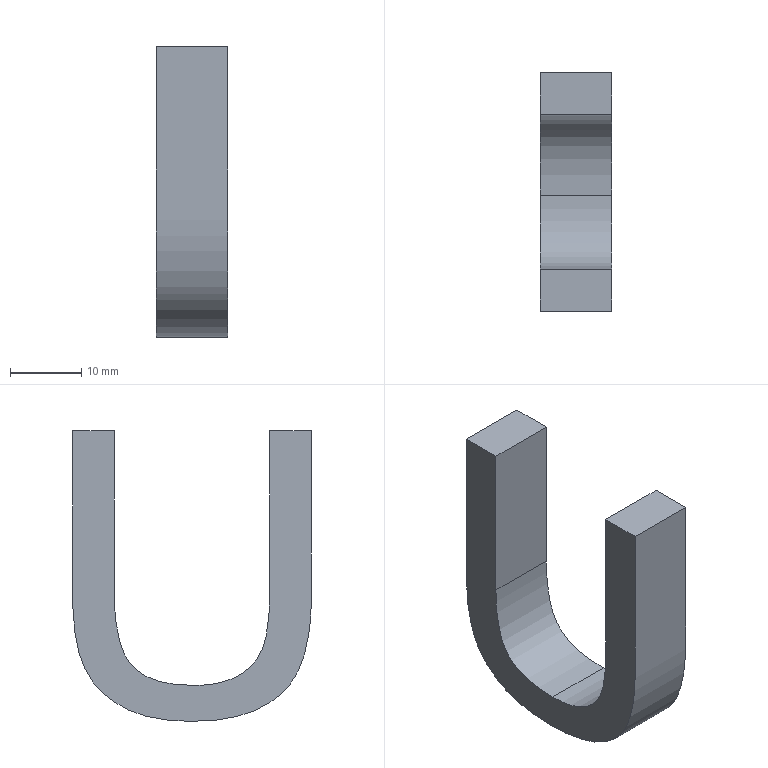Part | NX | features solid 2 | 1 solid | 8 faces | box 10 x 33.468 x 40.78 mm | volume 5118 mm3 | plane 5 | spline 3
STEP:
#1=CARTESIAN_POINT('',(2250.,262.21,377.01));
#2=VERTEX_POINT('',#1);
#3=CARTESIAN_POINT('',(2250.,262.21,400.));
#4=VERTEX_POINT('',#3);
#5=CARTESIAN_POINT('',(2250.,262.21,377.01));
#6=CARTESIAN_POINT('',(2250.,262.21,384.673));
#7=CARTESIAN_POINT('',(2250.,262.21,392.337));
#8=CARTESIAN_POINT('',(2250.,262.21,400.));
#9=B_SPLINE_CURVE_WITH_KNOTS('',3,(#5,#6,#7,#8),.UNSPECIFIED.,.F.,.F.,(4,4),(0.,0.1078),.PIECEWISE_BEZIER_KNOTS.);
#10=EDGE_CURVE('',#2,#4,#9,.T.);
#11=ORIENTED_EDGE('',*,*,#10,.F.);
#12=CARTESIAN_POINT('',(2260.,262.21,377.01));
#13=VERTEX_POINT('',#12);
#14=CARTESIAN_POINT('',(2260.,262.21,377.01));
#15=DIRECTION('',(-1.,0.,0.));
#16=VECTOR('',#15,1000.);
#17=LINE('',#14,#16);
#18=EDGE_CURVE('',#13,#2,#17,.T.);
#19=ORIENTED_EDGE('',*,*,#18,.F.);
#20=CARTESIAN_POINT('',(2260.,262.21,400.));
#21=VERTEX_POINT('',#20);
#22=CARTESIAN_POINT('',(2260.,262.21,377.01));
#23=CARTESIAN_POINT('',(2260.,262.21,384.673));
#24=CARTESIAN_POINT('',(2260.,262.21,392.337));
#25=CARTESIAN_POINT('',(2260.,262.21,400.));
#26=B_SPLINE_CURVE_WITH_KNOTS('',3,(#22,#23,#24,#25),.UNSPECIFIED.,.F.,.F.,(4,4),(0.,0.1078),.PIECEWISE_BEZIER_KNOTS.);
#27=EDGE_CURVE('',#13,#21,#26,.T.);
#28=ORIENTED_EDGE('',*,*,#27,.T.);
#29=CARTESIAN_POINT('',(2260.,262.21,400.));
#30=DIRECTION('',(-1.,0.,0.));
#31=VECTOR('',#30,1000.);
#32=LINE('',#29,#31);
#33=EDGE_CURVE('',#21,#4,#32,.T.);
#34=ORIENTED_EDGE('',*,*,#33,.T.);
#35=EDGE_LOOP('',(#11,#19,#28,#34));
#36=FACE_BOUND('',#35,.T.);
#37=CARTESIAN_POINT('',(2260.,262.21,377.01));
#38=DIRECTION('',(0.,-1.,0.));
#39=DIRECTION('',(0.,0.,-1.));
#40=AXIS2_PLACEMENT_3D('',#37,#38,#39);
#41=PLANE('',#40);
#42=ADVANCED_FACE('',(#36),#41,.T.);
#43=CARTESIAN_POINT('',(2250.,268.068,400.));
#44=VERTEX_POINT('',#43);
#45=CARTESIAN_POINT('',(2250.,262.21,400.));
#46=CARTESIAN_POINT('',(2250.,264.163,400.));
#47=CARTESIAN_POINT('',(2250.,266.116,400.));
#48=CARTESIAN_POINT('',(2250.,268.068,400.));
#49=B_SPLINE_CURVE_WITH_KNOTS('',3,(#45,#46,#47,#48),.UNSPECIFIED.,.F.,.F.,(4,4),(0.1078,0.1353),.PIECEWISE_BEZIER_KNOTS.);
#50=EDGE_CURVE('',#4,#44,#49,.T.);
#51=ORIENTED_EDGE('',*,*,#50,.F.);
#52=ORIENTED_EDGE('',*,*,#33,.F.);
#53=CARTESIAN_POINT('',(2260.,268.068,400.));
#54=VERTEX_POINT('',#53);
#55=CARTESIAN_POINT('',(2260.,262.21,400.));
#56=CARTESIAN_POINT('',(2260.,264.163,400.));
#57=CARTESIAN_POINT('',(2260.,266.116,400.));
#58=CARTESIAN_POINT('',(2260.,268.068,400.));
#59=B_SPLINE_CURVE_WITH_KNOTS('',3,(#55,#56,#57,#58),.UNSPECIFIED.,.F.,.F.,(4,4),(0.1078,0.1353),.PIECEWISE_BEZIER_KNOTS.);
#60=EDGE_CURVE('',#21,#54,#59,.T.);
#61=ORIENTED_EDGE('',*,*,#60,.T.);
#62=CARTESIAN_POINT('',(2260.,268.068,400.));
#63=DIRECTION('',(-1.,0.,0.));
#64=VECTOR('',#63,1000.);
#65=LINE('',#62,#64);
#66=EDGE_CURVE('',#54,#44,#65,.T.);
#67=ORIENTED_EDGE('',*,*,#66,.T.);
#68=EDGE_LOOP('',(#51,#52,#61,#67));
#69=FACE_BOUND('',#68,.T.);
#70=CARTESIAN_POINT('',(2260.,262.21,400.));
#71=DIRECTION('',(0.,0.,1.));
#72=DIRECTION('',(1.,0.,0.));
#73=AXIS2_PLACEMENT_3D('',#70,#71,#72);
#74=PLANE('',#73);
#75=ADVANCED_FACE('',(#69),#74,.T.);
#76=CARTESIAN_POINT('',(2250.,234.6,400.));
#77=VERTEX_POINT('',#76);
#78=CARTESIAN_POINT('',(2250.,268.068,400.));
#79=CARTESIAN_POINT('',(2250.,268.068,392.27));
#80=CARTESIAN_POINT('',(2250.,268.068,384.54));
#81=CARTESIAN_POINT('',(2250.,268.068,372.757));
#82=CARTESIAN_POINT('',(2250.,267.594,369.56));
#83=CARTESIAN_POINT('',(2250.,265.654,364.817));
#84=CARTESIAN_POINT('',(2250.,263.908,362.876));
#85=CARTESIAN_POINT('',(2250.,261.379,361.404));
#86=CARTESIAN_POINT('',(2250.,258.86,359.939));
#87=CARTESIAN_POINT('',(2250.,255.541,359.22));
#88=CARTESIAN_POINT('',(2250.,247.464,359.22));
#89=CARTESIAN_POINT('',(2250.,244.191,359.847));
#90=CARTESIAN_POINT('',(2250.,239.131,362.423));
#91=CARTESIAN_POINT('',(2250.,237.323,364.283));
#92=CARTESIAN_POINT('',(2250.,235.142,369.189));
#93=CARTESIAN_POINT('',(2250.,234.6,372.543));
#94=CARTESIAN_POINT('',(2250.,234.6,384.54));
#95=CARTESIAN_POINT('',(2250.,234.6,392.27));
#96=CARTESIAN_POINT('',(2250.,234.6,400.));
#97=B_SPLINE_CURVE_WITH_KNOTS('',3,(#78,#79,#80,#81,#82,#83,#84,#85,#86,#87,#88,#89,#90,#91,#92,#93,#94,#95,#96),.UNSPECIFIED.,.F.,.F.,(4,2,2,3,2,2,2,2,4),(0.1353,0.244,0.3011,0.3589,0.4118,0.4631,0.5147,0.5652,0.6568),.UNSPECIFIED.);
#98=EDGE_CURVE('',#44,#77,#97,.T.);
#99=ORIENTED_EDGE('',*,*,#98,.F.);
#100=ORIENTED_EDGE('',*,*,#66,.F.);
#101=CARTESIAN_POINT('',(2260.,234.6,400.));
#102=VERTEX_POINT('',#101);
#103=CARTESIAN_POINT('',(2260.,268.068,400.));
#104=CARTESIAN_POINT('',(2260.,268.068,392.27));
#105=CARTESIAN_POINT('',(2260.,268.068,384.54));
#106=CARTESIAN_POINT('',(2260.,268.068,372.757));
#107=CARTESIAN_POINT('',(2260.,267.594,369.56));
#108=CARTESIAN_POINT('',(2260.,265.654,364.817));
#109=CARTESIAN_POINT('',(2260.,263.908,362.876));
#110=CARTESIAN_POINT('',(2260.,261.379,361.404));
#111=CARTESIAN_POINT('',(2260.,258.86,359.939));
#112=CARTESIAN_POINT('',(2260.,255.541,359.22));
#113=CARTESIAN_POINT('',(2260.,247.464,359.22));
#114=CARTESIAN_POINT('',(2260.,244.191,359.847));
#115=CARTESIAN_POINT('',(2260.,239.131,362.423));
#116=CARTESIAN_POINT('',(2260.,237.323,364.283));
#117=CARTESIAN_POINT('',(2260.,235.142,369.189));
#118=CARTESIAN_POINT('',(2260.,234.6,372.543));
#119=CARTESIAN_POINT('',(2260.,234.6,384.54));
#120=CARTESIAN_POINT('',(2260.,234.6,392.27));
#121=CARTESIAN_POINT('',(2260.,234.6,400.));
#122=B_SPLINE_CURVE_WITH_KNOTS('',3,(#103,#104,#105,#106,#107,#108,#109,#110,#111,#112,#113,#114,#115,#116,#117,#118,#119,#120,#121),.UNSPECIFIED.,.F.,.F.,(4,2,2,3,2,2,2,2,4),(0.1353,0.244,0.3011,0.3589,0.4118,0.4631,0.5147,0.5652,0.6568),.UNSPECIFIED.);
#123=EDGE_CURVE('',#54,#102,#122,.T.);
#124=ORIENTED_EDGE('',*,*,#123,.T.);
#125=CARTESIAN_POINT('',(2260.,234.6,400.));
#126=DIRECTION('',(-1.,0.,0.));
#127=VECTOR('',#126,1000.);
#128=LINE('',#125,#127);
#129=EDGE_CURVE('',#102,#77,#128,.T.);
#130=ORIENTED_EDGE('',*,*,#129,.T.);
#131=EDGE_LOOP('',(#99,#100,#124,#130));
#132=FACE_BOUND('',#131,.T.);
#133=CARTESIAN_POINT('',(2260.,268.068,400.));
#134=CARTESIAN_POINT('',(2250.,268.068,400.));
#135=CARTESIAN_POINT('',(2260.,268.068,397.683));
#136=CARTESIAN_POINT('',(2250.,268.068,397.683));
#137=CARTESIAN_POINT('',(2260.,268.067,393.052));
#138=CARTESIAN_POINT('',(2250.,268.067,393.052));
#139=CARTESIAN_POINT('',(2260.,268.073,386.091));
#140=CARTESIAN_POINT('',(2250.,268.073,386.091));
#141=CARTESIAN_POINT('',(2260.,268.054,380.332));
#142=CARTESIAN_POINT('',(2250.,268.054,380.332));
#143=CARTESIAN_POINT('',(2260.,268.093,375.632));
#144=CARTESIAN_POINT('',(2250.,268.093,375.632));
#145=CARTESIAN_POINT('',(2260.,267.838,371.45));
#146=CARTESIAN_POINT('',(2250.,267.838,371.45));
#147=CARTESIAN_POINT('',(2260.,267.121,368.135));
#148=CARTESIAN_POINT('',(2250.,267.121,368.135));
#149=CARTESIAN_POINT('',(2260.,265.887,365.578));
#150=CARTESIAN_POINT('',(2250.,265.887,365.578));
#151=CARTESIAN_POINT('',(2260.,264.566,363.831));
#152=CARTESIAN_POINT('',(2250.,264.566,363.831));
#153=CARTESIAN_POINT('',(2260.,262.884,362.329));
#154=CARTESIAN_POINT('',(2250.,262.884,362.329));
#155=CARTESIAN_POINT('',(2260.,260.817,360.993));
#156=CARTESIAN_POINT('',(2250.,260.817,360.993));
#157=CARTESIAN_POINT('',(2260.,258.084,359.941));
#158=CARTESIAN_POINT('',(2250.,258.084,359.941));
#159=CARTESIAN_POINT('',(2260.,254.99,359.343));
#160=CARTESIAN_POINT('',(2250.,254.99,359.343));
#161=CARTESIAN_POINT('',(2260.,251.302,359.155));
#162=CARTESIAN_POINT('',(2250.,251.302,359.155));
#163=CARTESIAN_POINT('',(2260.,246.456,359.428));
#164=CARTESIAN_POINT('',(2250.,246.456,359.428));
#165=CARTESIAN_POINT('',(2260.,241.665,360.738));
#166=CARTESIAN_POINT('',(2250.,241.665,360.738));
#167=CARTESIAN_POINT('',(2260.,237.61,363.842));
#168=CARTESIAN_POINT('',(2250.,237.61,363.842));
#169=CARTESIAN_POINT('',(2260.,235.713,367.487));
#170=CARTESIAN_POINT('',(2250.,235.713,367.487));
#171=CARTESIAN_POINT('',(2260.,234.866,371.555));
#172=CARTESIAN_POINT('',(2250.,234.866,371.555));
#173=CARTESIAN_POINT('',(2260.,234.568,375.18));
#174=CARTESIAN_POINT('',(2250.,234.568,375.18));
#175=CARTESIAN_POINT('',(2260.,234.608,379.375));
#176=CARTESIAN_POINT('',(2250.,234.608,379.375));
#177=CARTESIAN_POINT('',(2260.,234.595,384.857));
#178=CARTESIAN_POINT('',(2250.,234.595,384.857));
#179=CARTESIAN_POINT('',(2260.,234.602,391.747));
#180=CARTESIAN_POINT('',(2250.,234.602,391.747));
#181=CARTESIAN_POINT('',(2260.,234.6,397.248));
#182=CARTESIAN_POINT('',(2250.,234.6,397.248));
#183=CARTESIAN_POINT('',(2260.,234.6,400.));
#184=CARTESIAN_POINT('',(2250.,234.6,400.));
#185=B_SPLINE_SURFACE_WITH_KNOTS('',3,1,((#133,#134),(#135,#136),(#137,#138),(#139,#140),(#141,#142),(#143,#144),(#145,#146),(#147,#148),(#149,#150),(#151,#152),(#153,#154),(#155,#156),(#157,#158),(#159,#160),(#161,#162),(#163,#164),(#165,#166),(#167,#168),(#169,#170),(#171,#172),(#173,#174),(#175,#176),(#177,#178),(#179,#180),(#181,#182),(#183,#184)),.SURF_OF_LINEAR_EXTRUSION.,.F.,.F.,.F.,(4,1,1,1,1,1,1,1,1,1,1,1,1,1,1,1,1,1,1,1,1,1,1,4),(2,2),(0.1353,0.1679,0.2005,0.2331,0.2494,0.2657,0.2983,0.3146,0.3309,0.3471,0.3634,0.3797,0.396,0.4123,0.4286,0.4612,0.4938,0.5264,0.5427,0.559,0.5753,0.5916,0.6242,0.6568),(0.,1.),.UNSPECIFIED.);
#186=ADVANCED_FACE('',(#132),#185,.T.);
#187=CARTESIAN_POINT('',(2250.,240.459,400.));
#188=VERTEX_POINT('',#187);
#189=CARTESIAN_POINT('',(2250.,234.6,400.));
#190=CARTESIAN_POINT('',(2250.,236.553,400.));
#191=CARTESIAN_POINT('',(2250.,238.506,400.));
#192=CARTESIAN_POINT('',(2250.,240.459,400.));
#193=B_SPLINE_CURVE_WITH_KNOTS('',3,(#189,#190,#191,#192),.UNSPECIFIED.,.F.,.F.,(4,4),(0.6568,0.686),.PIECEWISE_BEZIER_KNOTS.);
#194=EDGE_CURVE('',#77,#188,#193,.T.);
#195=ORIENTED_EDGE('',*,*,#194,.F.);
#196=ORIENTED_EDGE('',*,*,#129,.F.);
#197=CARTESIAN_POINT('',(2260.,240.459,400.));
#198=VERTEX_POINT('',#197);
#199=CARTESIAN_POINT('',(2260.,234.6,400.));
#200=CARTESIAN_POINT('',(2260.,236.553,400.));
#201=CARTESIAN_POINT('',(2260.,238.506,400.));
#202=CARTESIAN_POINT('',(2260.,240.459,400.));
#203=B_SPLINE_CURVE_WITH_KNOTS('',3,(#199,#200,#201,#202),.UNSPECIFIED.,.F.,.F.,(4,4),(0.6568,0.686),.PIECEWISE_BEZIER_KNOTS.);
#204=EDGE_CURVE('',#102,#198,#203,.T.);
#205=ORIENTED_EDGE('',*,*,#204,.T.);
#206=CARTESIAN_POINT('',(2260.,240.459,400.));
#207=DIRECTION('',(-1.,0.,0.));
#208=VECTOR('',#207,1000.);
#209=LINE('',#206,#208);
#210=EDGE_CURVE('',#198,#188,#209,.T.);
#211=ORIENTED_EDGE('',*,*,#210,.T.);
#212=EDGE_LOOP('',(#195,#196,#205,#211));
#213=FACE_BOUND('',#212,.T.);
#214=CARTESIAN_POINT('',(2260.,234.6,400.));
#215=DIRECTION('',(0.,0.,1.));
#216=DIRECTION('',(1.,0.,0.));
#217=AXIS2_PLACEMENT_3D('',#214,#215,#216);
#218=PLANE('',#217);
#219=ADVANCED_FACE('',(#213),#218,.T.);
#220=CARTESIAN_POINT('',(2250.,250.937,364.268));
#221=VERTEX_POINT('',#220);
#222=CARTESIAN_POINT('',(2250.,240.459,400.));
#223=CARTESIAN_POINT('',(2250.,240.459,392.337));
#224=CARTESIAN_POINT('',(2250.,240.459,384.673));
#225=CARTESIAN_POINT('',(2250.,240.459,373.537));
#226=CARTESIAN_POINT('',(2250.,240.795,370.983));
#227=CARTESIAN_POINT('',(2250.,241.471,369.356));
#228=CARTESIAN_POINT('',(2250.,242.156,367.709));
#229=CARTESIAN_POINT('',(2250.,243.304,366.455));
#230=CARTESIAN_POINT('',(2250.,246.583,364.692));
#231=CARTESIAN_POINT('',(2250.,248.581,364.237));
#232=CARTESIAN_POINT('',(2250.,250.937,364.268));
#233=B_SPLINE_CURVE_WITH_KNOTS('',3,(#222,#223,#224,#225,#226,#227,#228,#229,#230,#231,#232),.UNSPECIFIED.,.F.,.F.,(4,2,3,2,4),(0.686,0.8008,0.8528,0.8793,0.9064),.UNSPECIFIED.);
#234=EDGE_CURVE('',#188,#221,#233,.T.);
#235=ORIENTED_EDGE('',*,*,#234,.F.);
#236=ORIENTED_EDGE('',*,*,#210,.F.);
#237=CARTESIAN_POINT('',(2260.,250.937,364.268));
#238=VERTEX_POINT('',#237);
#239=CARTESIAN_POINT('',(2260.,240.459,400.));
#240=CARTESIAN_POINT('',(2260.,240.459,392.337));
#241=CARTESIAN_POINT('',(2260.,240.459,384.673));
#242=CARTESIAN_POINT('',(2260.,240.459,373.537));
#243=CARTESIAN_POINT('',(2260.,240.795,370.983));
#244=CARTESIAN_POINT('',(2260.,241.471,369.356));
#245=CARTESIAN_POINT('',(2260.,242.156,367.709));
#246=CARTESIAN_POINT('',(2260.,243.304,366.455));
#247=CARTESIAN_POINT('',(2260.,246.583,364.692));
#248=CARTESIAN_POINT('',(2260.,248.581,364.237));
#249=CARTESIAN_POINT('',(2260.,250.937,364.268));
#250=B_SPLINE_CURVE_WITH_KNOTS('',3,(#239,#240,#241,#242,#243,#244,#245,#246,#247,#248,#249),.UNSPECIFIED.,.F.,.F.,(4,2,3,2,4),(0.686,0.8008,0.8528,0.8793,0.9064),.UNSPECIFIED.);
#251=EDGE_CURVE('',#198,#238,#250,.T.);
#252=ORIENTED_EDGE('',*,*,#251,.T.);
#253=CARTESIAN_POINT('',(2260.,250.937,364.268));
#254=DIRECTION('',(-1.,0.,0.));
#255=VECTOR('',#254,1000.);
#256=LINE('',#253,#255);
#257=EDGE_CURVE('',#238,#221,#256,.T.);
#258=ORIENTED_EDGE('',*,*,#257,.T.);
#259=EDGE_LOOP('',(#235,#236,#252,#258));
#260=FACE_BOUND('',#259,.T.);
#261=CARTESIAN_POINT('',(2260.,240.459,400.));
#262=CARTESIAN_POINT('',(2250.,240.459,400.));
#263=CARTESIAN_POINT('',(2260.,240.459,398.161));
#264=CARTESIAN_POINT('',(2250.,240.459,398.161));
#265=CARTESIAN_POINT('',(2260.,240.459,394.484));
#266=CARTESIAN_POINT('',(2250.,240.459,394.484));
#267=CARTESIAN_POINT('',(2260.,240.458,388.967));
#268=CARTESIAN_POINT('',(2250.,240.458,388.967));
#269=CARTESIAN_POINT('',(2260.,240.459,383.453));
#270=CARTESIAN_POINT('',(2250.,240.459,383.453));
#271=CARTESIAN_POINT('',(2260.,240.456,378.849));
#272=CARTESIAN_POINT('',(2250.,240.456,378.849));
#273=CARTESIAN_POINT('',(2260.,240.462,375.187));
#274=CARTESIAN_POINT('',(2250.,240.462,375.187));
#275=CARTESIAN_POINT('',(2260.,240.604,373.276));
#276=CARTESIAN_POINT('',(2250.,240.604,373.276));
#277=CARTESIAN_POINT('',(2260.,240.785,371.929));
#278=CARTESIAN_POINT('',(2250.,240.785,371.929));
#279=CARTESIAN_POINT('',(2260.,240.956,371.019));
#280=CARTESIAN_POINT('',(2250.,240.956,371.019));
#281=CARTESIAN_POINT('',(2260.,241.13,370.338));
#282=CARTESIAN_POINT('',(2250.,241.13,370.338));
#283=CARTESIAN_POINT('',(2260.,241.283,369.85));
#284=CARTESIAN_POINT('',(2250.,241.283,369.85));
#285=CARTESIAN_POINT('',(2260.,241.395,369.545));
#286=CARTESIAN_POINT('',(2250.,241.395,369.545));
#287=CARTESIAN_POINT('',(2260.,241.467,369.361));
#288=CARTESIAN_POINT('',(2250.,241.467,369.361));
#289=CARTESIAN_POINT('',(2260.,241.679,368.88));
#290=CARTESIAN_POINT('',(2250.,241.679,368.88));
#291=CARTESIAN_POINT('',(2260.,242.034,368.217));
#292=CARTESIAN_POINT('',(2250.,242.034,368.217));
#293=CARTESIAN_POINT('',(2260.,242.946,366.927));
#294=CARTESIAN_POINT('',(2250.,242.946,366.927));
#295=CARTESIAN_POINT('',(2260.,244.726,365.527));
#296=CARTESIAN_POINT('',(2250.,244.726,365.527));
#297=CARTESIAN_POINT('',(2260.,247.533,364.47));
#298=CARTESIAN_POINT('',(2250.,247.533,364.47));
#299=CARTESIAN_POINT('',(2260.,249.738,364.252));
#300=CARTESIAN_POINT('',(2250.,249.738,364.252));
#301=CARTESIAN_POINT('',(2260.,250.937,364.268));
#302=CARTESIAN_POINT('',(2250.,250.937,364.268));
#303=B_SPLINE_SURFACE_WITH_KNOTS('',3,1,((#261,#262),(#263,#264),(#265,#266),(#267,#268),(#269,#270),(#271,#272),(#273,#274),(#275,#276),(#277,#278),(#279,#280),(#281,#282),(#283,#284),(#285,#286),(#287,#288),(#289,#290),(#291,#292),(#293,#294),(#295,#296),(#297,#298),(#299,#300),(#301,#302)),.SURF_OF_LINEAR_EXTRUSION.,.F.,.F.,.F.,(4,1,1,1,1,1,1,1,1,1,1,1,1,1,1,1,1,1,4),(2,2),(0.686,0.7136,0.7411,0.7687,0.7962,0.81,0.8237,0.8306,0.8375,0.8444,0.8478,0.8513,0.853,0.8547,0.8582,0.8651,0.8788,0.8926,0.9064),(0.,1.),.UNSPECIFIED.);
#304=ADVANCED_FACE('',(#260),#303,.T.);
#305=CARTESIAN_POINT('',(2250.,250.937,364.268));
#306=CARTESIAN_POINT('',(2250.,255.021,364.237));
#307=CARTESIAN_POINT('',(2250.,257.896,365.109));
#308=CARTESIAN_POINT('',(2250.,261.338,368.642));
#309=CARTESIAN_POINT('',(2250.,262.21,372.008));
#310=CARTESIAN_POINT('',(2250.,262.21,377.01));
#311=B_SPLINE_CURVE_WITH_KNOTS('',3,(#305,#306,#307,#308,#309,#310),.UNSPECIFIED.,.F.,.F.,(4,2,4),(0.9064,0.9534,1.),.UNSPECIFIED.);
#312=EDGE_CURVE('',#221,#2,#311,.T.);
#313=ORIENTED_EDGE('',*,*,#312,.F.);
#314=ORIENTED_EDGE('',*,*,#257,.F.);
#315=CARTESIAN_POINT('',(2260.,250.937,364.268));
#316=CARTESIAN_POINT('',(2260.,255.021,364.237));
#317=CARTESIAN_POINT('',(2260.,257.896,365.109));
#318=CARTESIAN_POINT('',(2260.,261.338,368.642));
#319=CARTESIAN_POINT('',(2260.,262.21,372.008));
#320=CARTESIAN_POINT('',(2260.,262.21,377.01));
#321=B_SPLINE_CURVE_WITH_KNOTS('',3,(#315,#316,#317,#318,#319,#320),.UNSPECIFIED.,.F.,.F.,(4,2,4),(0.9064,0.9534,1.),.UNSPECIFIED.);
#322=EDGE_CURVE('',#238,#13,#321,.T.);
#323=ORIENTED_EDGE('',*,*,#322,.T.);
#324=ORIENTED_EDGE('',*,*,#18,.T.);
#325=EDGE_LOOP('',(#313,#314,#323,#324));
#326=FACE_BOUND('',#325,.T.);
#327=CARTESIAN_POINT('',(2260.,250.937,364.268));
#328=CARTESIAN_POINT('',(2250.,250.937,364.268));
#329=CARTESIAN_POINT('',(2260.,252.97,364.252));
#330=CARTESIAN_POINT('',(2250.,252.97,364.252));
#331=CARTESIAN_POINT('',(2260.,255.569,364.562));
#332=CARTESIAN_POINT('',(2250.,255.569,364.562));
#333=CARTESIAN_POINT('',(2260.,258.164,365.659));
#334=CARTESIAN_POINT('',(2250.,258.164,365.659));
#335=CARTESIAN_POINT('',(2260.,259.665,366.783));
#336=CARTESIAN_POINT('',(2250.,259.665,366.783));
#337=CARTESIAN_POINT('',(2260.,260.79,368.371));
#338=CARTESIAN_POINT('',(2250.,260.79,368.371));
#339=CARTESIAN_POINT('',(2260.,261.882,371.353));
#340=CARTESIAN_POINT('',(2250.,261.882,371.353));
#341=CARTESIAN_POINT('',(2260.,262.21,374.498));
#342=CARTESIAN_POINT('',(2250.,262.21,374.498));
#343=CARTESIAN_POINT('',(2260.,262.21,377.01));
#344=CARTESIAN_POINT('',(2250.,262.21,377.01));
#345=B_SPLINE_SURFACE_WITH_KNOTS('',3,1,((#327,#328),(#329,#330),(#331,#332),(#333,#334),(#335,#336),(#337,#338),(#339,#340),(#341,#342),(#343,#344)),.SURF_OF_LINEAR_EXTRUSION.,.F.,.F.,.F.,(4,1,1,1,1,1,4),(2,2),(0.9064,0.9298,0.9415,0.9532,0.9649,0.9766,1.),(0.,1.),.UNSPECIFIED.);
#346=ADVANCED_FACE('',(#326),#345,.T.);
#347=ORIENTED_EDGE('',*,*,#27,.F.);
#348=ORIENTED_EDGE('',*,*,#322,.F.);
#349=ORIENTED_EDGE('',*,*,#251,.F.);
#350=ORIENTED_EDGE('',*,*,#204,.F.);
#351=ORIENTED_EDGE('',*,*,#123,.F.);
#352=ORIENTED_EDGE('',*,*,#60,.F.);
#353=EDGE_LOOP('',(#347,#348,#349,#350,#351,#352));
#354=FACE_BOUND('',#353,.T.);
#355=CARTESIAN_POINT('',(2260.,254.891,359.411));
#356=DIRECTION('',(1.,0.,0.));
#357=DIRECTION('',(0.,1.,0.));
#358=AXIS2_PLACEMENT_3D('',#355,#356,#357);
#359=PLANE('',#358);
#360=ADVANCED_FACE('',(#354),#359,.T.);
#361=ORIENTED_EDGE('',*,*,#10,.T.);
#362=ORIENTED_EDGE('',*,*,#50,.T.);
#363=ORIENTED_EDGE('',*,*,#98,.T.);
#364=ORIENTED_EDGE('',*,*,#194,.T.);
#365=ORIENTED_EDGE('',*,*,#234,.T.);
#366=ORIENTED_EDGE('',*,*,#312,.T.);
#367=EDGE_LOOP('',(#361,#362,#363,#364,#365,#366));
#368=FACE_BOUND('',#367,.T.);
#369=CARTESIAN_POINT('',(2250.,254.891,359.411));
#370=DIRECTION('',(1.,0.,0.));
#371=DIRECTION('',(0.,1.,0.));
#372=AXIS2_PLACEMENT_3D('',#369,#370,#371);
#373=PLANE('',#372);
#374=ADVANCED_FACE('',(#368),#373,.F.);
#375=CLOSED_SHELL('',(#42,#75,#186,#219,#304,#346,#360,#374));
#376=MANIFOLD_SOLID_BREP('',#375);
#377=(LENGTH_UNIT()NAMED_UNIT(*)SI_UNIT(.MILLI.,.METRE.));
#378=UNCERTAINTY_MEASURE_WITH_UNIT(LENGTH_MEASURE(0.0508),#377,'','');
#379=(NAMED_UNIT(*)PLANE_ANGLE_UNIT()SI_UNIT($,.RADIAN.));
#380=(NAMED_UNIT(*)SI_UNIT($,.STERADIAN.)SOLID_ANGLE_UNIT());
#381=(GEOMETRIC_REPRESENTATION_CONTEXT(3)GLOBAL_UNCERTAINTY_ASSIGNED_CONTEXT((#378))GLOBAL_UNIT_ASSIGNED_CONTEXT((#377,#379,#380))REPRESENTATION_CONTEXT('',''));
#382=ADVANCED_BREP_SHAPE_REPRESENTATION('',(#376),#381);